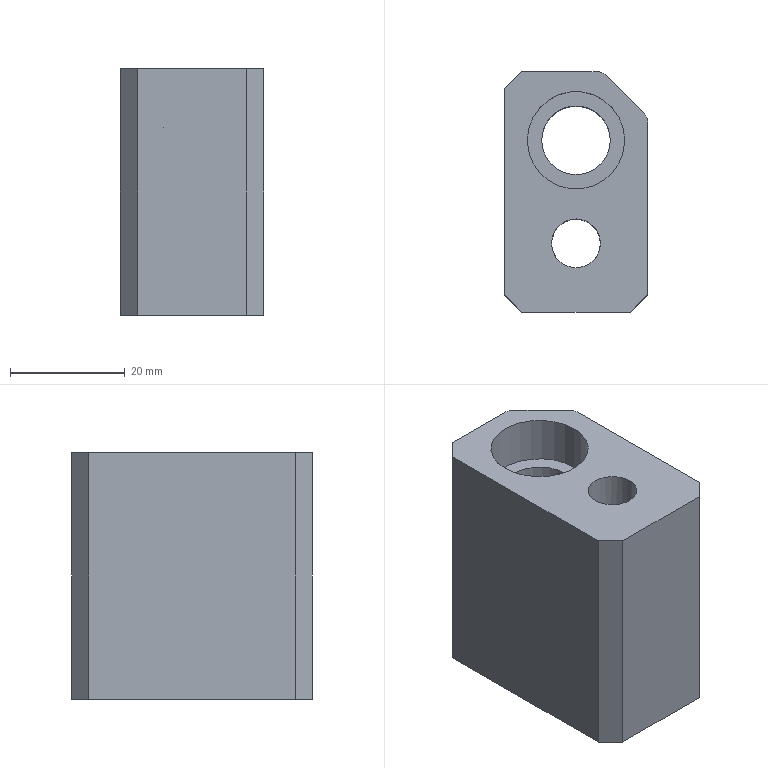Part | NX | features PH-5 2 | 1 solid | 18 faces | box 25 x 42 x 43 mm | volume 33756 mm3 | plane 12 | cylinder 6 | commonest cylinder face diameters 4 x2 8.5 x1 12.001 x1 14.5 x1 17 x1
STEP:
#1=CARTESIAN_POINT('',(2467.597,-809.449,945.716));
#2=VERTEX_POINT('',#1);
#3=CARTESIAN_POINT('',(2459.097,-809.449,945.716));
#4=DIRECTION('',(0.,0.,1.));
#5=DIRECTION('',(1.,0.,0.));
#6=AXIS2_PLACEMENT_3D('',#3,#4,#5);
#7=CIRCLE('',#6,8.5);
#8=EDGE_CURVE('',#2,#2,#7,.F.);
#9=ORIENTED_EDGE('',*,*,#8,.T.);
#10=EDGE_LOOP('',(#9));
#11=FACE_BOUND('',#10,.T.);
#12=CARTESIAN_POINT('',(2459.097,-831.699,945.716));
#13=VERTEX_POINT('',#12);
#14=CARTESIAN_POINT('',(2459.097,-827.449,945.716));
#15=DIRECTION('',(0.,0.,1.));
#16=DIRECTION('',(0.,-1.,0.));
#17=AXIS2_PLACEMENT_3D('',#14,#15,#16);
#18=CIRCLE('',#17,4.25);
#19=EDGE_CURVE('',#13,#13,#18,.T.);
#20=ORIENTED_EDGE('',*,*,#19,.F.);
#21=EDGE_LOOP('',(#20));
#22=FACE_BOUND('',#21,.T.);
#23=CARTESIAN_POINT('',(2471.011,-804.863,945.716));
#24=VERTEX_POINT('',#23);
#25=CARTESIAN_POINT('',(2464.183,-798.035,945.716));
#26=VERTEX_POINT('',#25);
#27=CARTESIAN_POINT('',(2472.347,-806.199,945.716));
#28=DIRECTION('',(0.7071,-0.7071,0.));
#29=VECTOR('',#28,1000.);
#30=LINE('',#27,#29);
#31=EDGE_CURVE('',#24,#26,#30,.F.);
#32=ORIENTED_EDGE('',*,*,#31,.T.);
#33=CARTESIAN_POINT('',(2462.769,-797.449,945.716));
#34=VERTEX_POINT('',#33);
#35=CARTESIAN_POINT('',(2462.769,-799.449,945.716));
#36=DIRECTION('',(0.,0.,1.));
#37=DIRECTION('',(1.,0.,0.));
#38=AXIS2_PLACEMENT_3D('',#35,#36,#37);
#39=CIRCLE('',#38,2.);
#40=EDGE_CURVE('',#26,#34,#39,.T.);
#41=ORIENTED_EDGE('',*,*,#40,.T.);
#42=CARTESIAN_POINT('',(2449.597,-797.449,945.716));
#43=VERTEX_POINT('',#42);
#44=CARTESIAN_POINT('',(2459.097,-797.449,945.716));
#45=DIRECTION('',(1.,0.,0.));
#46=VECTOR('',#45,1000.);
#47=LINE('',#44,#46);
#48=EDGE_CURVE('',#43,#34,#47,.T.);
#49=ORIENTED_EDGE('',*,*,#48,.F.);
#50=CARTESIAN_POINT('',(2446.597,-800.449,945.716));
#51=VERTEX_POINT('',#50);
#52=CARTESIAN_POINT('',(2443.347,-803.699,945.716));
#53=DIRECTION('',(0.7071,0.7071,0.));
#54=VECTOR('',#53,1000.);
#55=LINE('',#52,#54);
#56=EDGE_CURVE('',#43,#51,#55,.F.);
#57=ORIENTED_EDGE('',*,*,#56,.T.);
#58=CARTESIAN_POINT('',(2446.597,-836.449,945.716));
#59=VERTEX_POINT('',#58);
#60=CARTESIAN_POINT('',(2446.597,-819.449,945.716));
#61=DIRECTION('',(0.,1.,0.));
#62=VECTOR('',#61,1000.);
#63=LINE('',#60,#62);
#64=EDGE_CURVE('',#59,#51,#63,.T.);
#65=ORIENTED_EDGE('',*,*,#64,.F.);
#66=CARTESIAN_POINT('',(2449.597,-839.449,945.716));
#67=VERTEX_POINT('',#66);
#68=CARTESIAN_POINT('',(2444.347,-834.199,945.716));
#69=DIRECTION('',(-0.7071,0.7071,0.));
#70=VECTOR('',#69,1000.);
#71=LINE('',#68,#70);
#72=EDGE_CURVE('',#59,#67,#71,.F.);
#73=ORIENTED_EDGE('',*,*,#72,.T.);
#74=CARTESIAN_POINT('',(2468.597,-839.449,945.716));
#75=VERTEX_POINT('',#74);
#76=CARTESIAN_POINT('',(2459.097,-839.449,945.716));
#77=DIRECTION('',(-1.,0.,0.));
#78=VECTOR('',#77,1000.);
#79=LINE('',#76,#78);
#80=EDGE_CURVE('',#75,#67,#79,.T.);
#81=ORIENTED_EDGE('',*,*,#80,.F.);
#82=CARTESIAN_POINT('',(2471.597,-836.449,945.716));
#83=VERTEX_POINT('',#82);
#84=CARTESIAN_POINT('',(2473.847,-834.199,945.716));
#85=DIRECTION('',(-0.7071,-0.7071,0.));
#86=VECTOR('',#85,1000.);
#87=LINE('',#84,#86);
#88=EDGE_CURVE('',#75,#83,#87,.F.);
#89=ORIENTED_EDGE('',*,*,#88,.T.);
#90=CARTESIAN_POINT('',(2471.597,-806.277,945.716));
#91=VERTEX_POINT('',#90);
#92=CARTESIAN_POINT('',(2471.597,-819.449,945.716));
#93=DIRECTION('',(0.,-1.,0.));
#94=VECTOR('',#93,1000.);
#95=LINE('',#92,#94);
#96=EDGE_CURVE('',#91,#83,#95,.T.);
#97=ORIENTED_EDGE('',*,*,#96,.F.);
#98=CARTESIAN_POINT('',(2469.597,-806.277,945.716));
#99=DIRECTION('',(0.,0.,1.));
#100=DIRECTION('',(1.,0.,0.));
#101=AXIS2_PLACEMENT_3D('',#98,#99,#100);
#102=CIRCLE('',#101,2.);
#103=EDGE_CURVE('',#91,#24,#102,.T.);
#104=ORIENTED_EDGE('',*,*,#103,.T.);
#105=EDGE_LOOP('',(#32,#41,#49,#57,#65,#73,#81,#89,#97,#104));
#106=FACE_BOUND('',#105,.T.);
#107=CARTESIAN_POINT('',(2459.097,-819.449,945.716));
#108=DIRECTION('',(0.,0.,1.));
#109=DIRECTION('',(-1.,0.,0.));
#110=AXIS2_PLACEMENT_3D('',#107,#108,#109);
#111=PLANE('',#110);
#112=ADVANCED_FACE('',(#11,#22,#106),#111,.T.);
#113=ORIENTED_EDGE('',*,*,#48,.T.);
#114=CARTESIAN_POINT('',(2462.769,-797.449,902.716));
#115=VERTEX_POINT('',#114);
#116=CARTESIAN_POINT('',(2462.769,-797.449,920.716));
#117=DIRECTION('',(0.,0.,1.));
#118=VECTOR('',#117,1000.);
#119=LINE('',#116,#118);
#120=EDGE_CURVE('',#34,#115,#119,.F.);
#121=ORIENTED_EDGE('',*,*,#120,.T.);
#122=CARTESIAN_POINT('',(2449.597,-797.449,902.716));
#123=VERTEX_POINT('',#122);
#124=CARTESIAN_POINT('',(2459.097,-797.449,902.716));
#125=DIRECTION('',(-1.,0.,0.));
#126=VECTOR('',#125,1000.);
#127=LINE('',#124,#126);
#128=EDGE_CURVE('',#115,#123,#127,.T.);
#129=ORIENTED_EDGE('',*,*,#128,.T.);
#130=CARTESIAN_POINT('',(2449.597,-797.449,920.716));
#131=DIRECTION('',(0.,0.,-1.));
#132=VECTOR('',#131,1000.);
#133=LINE('',#130,#132);
#134=EDGE_CURVE('',#123,#43,#133,.F.);
#135=ORIENTED_EDGE('',*,*,#134,.T.);
#136=EDGE_LOOP('',(#113,#121,#129,#135));
#137=FACE_BOUND('',#136,.T.);
#138=CARTESIAN_POINT('',(2459.097,-797.449,920.716));
#139=DIRECTION('',(0.,1.,0.));
#140=DIRECTION('',(0.,0.,-1.));
#141=AXIS2_PLACEMENT_3D('',#138,#139,#140);
#142=PLANE('',#141);
#143=ADVANCED_FACE('',(#137),#142,.T.);
#144=CARTESIAN_POINT('',(2471.597,-836.449,902.716));
#145=VERTEX_POINT('',#144);
#146=CARTESIAN_POINT('',(2471.597,-806.277,902.716));
#147=VERTEX_POINT('',#146);
#148=CARTESIAN_POINT('',(2471.597,-819.449,902.716));
#149=DIRECTION('',(0.,1.,0.));
#150=VECTOR('',#149,1000.);
#151=LINE('',#148,#150);
#152=EDGE_CURVE('',#145,#147,#151,.T.);
#153=ORIENTED_EDGE('',*,*,#152,.T.);
#154=CARTESIAN_POINT('',(2471.597,-806.277,920.716));
#155=DIRECTION('',(0.,0.,-1.));
#156=VECTOR('',#155,1000.);
#157=LINE('',#154,#156);
#158=EDGE_CURVE('',#147,#91,#157,.F.);
#159=ORIENTED_EDGE('',*,*,#158,.T.);
#160=ORIENTED_EDGE('',*,*,#96,.T.);
#161=CARTESIAN_POINT('',(2471.597,-836.449,920.716));
#162=DIRECTION('',(0.,0.,-1.));
#163=VECTOR('',#162,1000.);
#164=LINE('',#161,#163);
#165=EDGE_CURVE('',#83,#145,#164,.T.);
#166=ORIENTED_EDGE('',*,*,#165,.T.);
#167=EDGE_LOOP('',(#153,#159,#160,#166));
#168=FACE_BOUND('',#167,.T.);
#169=CARTESIAN_POINT('',(2471.597,-819.449,920.716));
#170=DIRECTION('',(1.,0.,0.));
#171=DIRECTION('',(0.,0.,1.));
#172=AXIS2_PLACEMENT_3D('',#169,#170,#171);
#173=PLANE('',#172);
#174=ADVANCED_FACE('',(#168),#173,.T.);
#175=CARTESIAN_POINT('',(2449.597,-839.449,902.716));
#176=VERTEX_POINT('',#175);
#177=CARTESIAN_POINT('',(2468.597,-839.449,902.716));
#178=VERTEX_POINT('',#177);
#179=CARTESIAN_POINT('',(2459.097,-839.449,902.716));
#180=DIRECTION('',(1.,0.,0.));
#181=VECTOR('',#180,1000.);
#182=LINE('',#179,#181);
#183=EDGE_CURVE('',#176,#178,#182,.T.);
#184=ORIENTED_EDGE('',*,*,#183,.T.);
#185=CARTESIAN_POINT('',(2468.597,-839.449,920.716));
#186=DIRECTION('',(0.,0.,1.));
#187=VECTOR('',#186,1000.);
#188=LINE('',#185,#187);
#189=EDGE_CURVE('',#178,#75,#188,.T.);
#190=ORIENTED_EDGE('',*,*,#189,.T.);
#191=ORIENTED_EDGE('',*,*,#80,.T.);
#192=CARTESIAN_POINT('',(2449.597,-839.449,920.716));
#193=DIRECTION('',(0.,0.,-1.));
#194=VECTOR('',#193,1000.);
#195=LINE('',#192,#194);
#196=EDGE_CURVE('',#67,#176,#195,.T.);
#197=ORIENTED_EDGE('',*,*,#196,.T.);
#198=EDGE_LOOP('',(#184,#190,#191,#197));
#199=FACE_BOUND('',#198,.T.);
#200=CARTESIAN_POINT('',(2459.097,-839.449,920.716));
#201=DIRECTION('',(0.,-1.,0.));
#202=DIRECTION('',(0.,0.,1.));
#203=AXIS2_PLACEMENT_3D('',#200,#201,#202);
#204=PLANE('',#203);
#205=ADVANCED_FACE('',(#199),#204,.T.);
#206=CARTESIAN_POINT('',(2453.097,-809.449,902.716));
#207=VERTEX_POINT('',#206);
#208=CARTESIAN_POINT('',(2459.097,-809.449,902.716));
#209=DIRECTION('',(0.,0.,-1.));
#210=DIRECTION('',(-1.,0.,0.));
#211=AXIS2_PLACEMENT_3D('',#208,#209,#210);
#212=CIRCLE('',#211,6.);
#213=EDGE_CURVE('',#207,#207,#212,.T.);
#214=ORIENTED_EDGE('',*,*,#213,.F.);
#215=EDGE_LOOP('',(#214));
#216=FACE_BOUND('',#215,.T.);
#217=CARTESIAN_POINT('',(2451.847,-827.449,902.716));
#218=VERTEX_POINT('',#217);
#219=CARTESIAN_POINT('',(2459.097,-827.449,902.716));
#220=DIRECTION('',(0.,0.,-1.));
#221=DIRECTION('',(-1.,0.,0.));
#222=AXIS2_PLACEMENT_3D('',#219,#220,#221);
#223=CIRCLE('',#222,7.25);
#224=EDGE_CURVE('',#218,#218,#223,.F.);
#225=ORIENTED_EDGE('',*,*,#224,.T.);
#226=EDGE_LOOP('',(#225));
#227=FACE_BOUND('',#226,.T.);
#228=ORIENTED_EDGE('',*,*,#128,.F.);
#229=CARTESIAN_POINT('',(2464.183,-798.035,902.716));
#230=VERTEX_POINT('',#229);
#231=CARTESIAN_POINT('',(2462.769,-799.449,902.716));
#232=DIRECTION('',(0.,0.,-1.));
#233=DIRECTION('',(-1.,0.,0.));
#234=AXIS2_PLACEMENT_3D('',#231,#232,#233);
#235=CIRCLE('',#234,2.);
#236=EDGE_CURVE('',#115,#230,#235,.T.);
#237=ORIENTED_EDGE('',*,*,#236,.T.);
#238=CARTESIAN_POINT('',(2471.011,-804.863,902.716));
#239=VERTEX_POINT('',#238);
#240=CARTESIAN_POINT('',(2472.347,-806.199,902.716));
#241=DIRECTION('',(-0.7071,0.7071,0.));
#242=VECTOR('',#241,1000.);
#243=LINE('',#240,#242);
#244=EDGE_CURVE('',#230,#239,#243,.F.);
#245=ORIENTED_EDGE('',*,*,#244,.T.);
#246=CARTESIAN_POINT('',(2469.597,-806.277,902.716));
#247=DIRECTION('',(0.,0.,-1.));
#248=DIRECTION('',(-1.,0.,0.));
#249=AXIS2_PLACEMENT_3D('',#246,#247,#248);
#250=CIRCLE('',#249,2.);
#251=EDGE_CURVE('',#239,#147,#250,.T.);
#252=ORIENTED_EDGE('',*,*,#251,.T.);
#253=ORIENTED_EDGE('',*,*,#152,.F.);
#254=CARTESIAN_POINT('',(2473.847,-834.199,902.716));
#255=DIRECTION('',(0.7071,0.7071,0.));
#256=VECTOR('',#255,1000.);
#257=LINE('',#254,#256);
#258=EDGE_CURVE('',#145,#178,#257,.F.);
#259=ORIENTED_EDGE('',*,*,#258,.T.);
#260=ORIENTED_EDGE('',*,*,#183,.F.);
#261=CARTESIAN_POINT('',(2446.597,-836.449,902.716));
#262=VERTEX_POINT('',#261);
#263=CARTESIAN_POINT('',(2444.347,-834.199,902.716));
#264=DIRECTION('',(0.7071,-0.7071,0.));
#265=VECTOR('',#264,1000.);
#266=LINE('',#263,#265);
#267=EDGE_CURVE('',#176,#262,#266,.F.);
#268=ORIENTED_EDGE('',*,*,#267,.T.);
#269=CARTESIAN_POINT('',(2446.597,-800.449,902.716));
#270=VERTEX_POINT('',#269);
#271=CARTESIAN_POINT('',(2446.597,-819.449,902.716));
#272=DIRECTION('',(0.,-1.,0.));
#273=VECTOR('',#272,1000.);
#274=LINE('',#271,#273);
#275=EDGE_CURVE('',#270,#262,#274,.T.);
#276=ORIENTED_EDGE('',*,*,#275,.F.);
#277=CARTESIAN_POINT('',(2443.347,-803.699,902.716));
#278=DIRECTION('',(-0.7071,-0.7071,0.));
#279=VECTOR('',#278,1000.);
#280=LINE('',#277,#279);
#281=EDGE_CURVE('',#270,#123,#280,.F.);
#282=ORIENTED_EDGE('',*,*,#281,.T.);
#283=EDGE_LOOP('',(#228,#237,#245,#252,#253,#259,#260,#268,#276,#282));
#284=FACE_BOUND('',#283,.T.);
#285=CARTESIAN_POINT('',(2459.097,-819.449,902.716));
#286=DIRECTION('',(0.,0.,-1.));
#287=DIRECTION('',(1.,0.,0.));
#288=AXIS2_PLACEMENT_3D('',#285,#286,#287);
#289=PLANE('',#288);
#290=ADVANCED_FACE('',(#216,#227,#284),#289,.T.);
#291=ORIENTED_EDGE('',*,*,#275,.T.);
#292=CARTESIAN_POINT('',(2446.597,-836.449,920.716));
#293=DIRECTION('',(0.,0.,1.));
#294=VECTOR('',#293,1000.);
#295=LINE('',#292,#294);
#296=EDGE_CURVE('',#262,#59,#295,.T.);
#297=ORIENTED_EDGE('',*,*,#296,.T.);
#298=ORIENTED_EDGE('',*,*,#64,.T.);
#299=CARTESIAN_POINT('',(2446.597,-800.449,920.716));
#300=DIRECTION('',(0.,0.,1.));
#301=VECTOR('',#300,1000.);
#302=LINE('',#299,#301);
#303=EDGE_CURVE('',#51,#270,#302,.F.);
#304=ORIENTED_EDGE('',*,*,#303,.T.);
#305=EDGE_LOOP('',(#291,#297,#298,#304));
#306=FACE_BOUND('',#305,.T.);
#307=CARTESIAN_POINT('',(2446.597,-819.449,920.716));
#308=DIRECTION('',(-1.,0.,0.));
#309=DIRECTION('',(0.,0.,-1.));
#310=AXIS2_PLACEMENT_3D('',#307,#308,#309);
#311=PLANE('',#310);
#312=ADVANCED_FACE('',(#306),#311,.T.);
#313=ORIENTED_EDGE('',*,*,#267,.F.);
#314=ORIENTED_EDGE('',*,*,#196,.F.);
#315=ORIENTED_EDGE('',*,*,#72,.F.);
#316=ORIENTED_EDGE('',*,*,#296,.F.);
#317=EDGE_LOOP('',(#313,#314,#315,#316));
#318=FACE_BOUND('',#317,.T.);
#319=CARTESIAN_POINT('',(2446.597,-836.449,920.716));
#320=DIRECTION('',(0.7071,0.7071,0.));
#321=DIRECTION('',(-0.7071,0.7071,0.));
#322=AXIS2_PLACEMENT_3D('',#319,#320,#321);
#323=PLANE('',#322);
#324=ADVANCED_FACE('',(#318),#323,.F.);
#325=ORIENTED_EDGE('',*,*,#281,.F.);
#326=ORIENTED_EDGE('',*,*,#303,.F.);
#327=ORIENTED_EDGE('',*,*,#56,.F.);
#328=ORIENTED_EDGE('',*,*,#134,.F.);
#329=EDGE_LOOP('',(#325,#326,#327,#328));
#330=FACE_BOUND('',#329,.T.);
#331=CARTESIAN_POINT('',(2449.597,-797.449,920.716));
#332=DIRECTION('',(0.7071,-0.7071,0.));
#333=DIRECTION('',(0.7071,0.7071,0.));
#334=AXIS2_PLACEMENT_3D('',#331,#332,#333);
#335=PLANE('',#334);
#336=ADVANCED_FACE('',(#330),#335,.F.);
#337=CARTESIAN_POINT('',(2463.347,-827.449,913.716));
#338=VERTEX_POINT('',#337);
#339=CARTESIAN_POINT('',(2459.097,-827.449,913.716));
#340=DIRECTION('',(0.,0.,1.));
#341=DIRECTION('',(1.,0.,0.));
#342=AXIS2_PLACEMENT_3D('',#339,#340,#341);
#343=CIRCLE('',#342,4.25);
#344=EDGE_CURVE('',#338,#338,#343,.T.);
#345=ORIENTED_EDGE('',*,*,#344,.T.);
#346=EDGE_LOOP('',(#345));
#347=FACE_BOUND('',#346,.T.);
#348=CARTESIAN_POINT('',(2466.347,-827.449,913.716));
#349=VERTEX_POINT('',#348);
#350=CARTESIAN_POINT('',(2459.097,-827.449,913.716));
#351=DIRECTION('',(0.,0.,1.));
#352=DIRECTION('',(1.,0.,0.));
#353=AXIS2_PLACEMENT_3D('',#350,#351,#352);
#354=CIRCLE('',#353,7.25);
#355=EDGE_CURVE('',#349,#349,#354,.T.);
#356=ORIENTED_EDGE('',*,*,#355,.F.);
#357=EDGE_LOOP('',(#356));
#358=FACE_BOUND('',#357,.T.);
#359=CARTESIAN_POINT('',(2459.097,-827.449,913.716));
#360=DIRECTION('',(0.,0.,1.));
#361=DIRECTION('',(0.,-1.,0.));
#362=AXIS2_PLACEMENT_3D('',#359,#360,#361);
#363=PLANE('',#362);
#364=ADVANCED_FACE('',(#347,#358),#363,.F.);
#365=ORIENTED_EDGE('',*,*,#224,.F.);
#366=EDGE_LOOP('',(#365));
#367=FACE_BOUND('',#366,.T.);
#368=ORIENTED_EDGE('',*,*,#355,.T.);
#369=EDGE_LOOP('',(#368));
#370=FACE_BOUND('',#369,.T.);
#371=CARTESIAN_POINT('',(2459.097,-827.449,931.716));
#372=DIRECTION('',(0.,0.,-1.));
#373=DIRECTION('',(-1.,0.,0.));
#374=AXIS2_PLACEMENT_3D('',#371,#372,#373);
#375=CYLINDRICAL_SURFACE('',#374,7.25);
#376=ADVANCED_FACE('',(#367,#370),#375,.F.);
#377=ORIENTED_EDGE('',*,*,#19,.T.);
#378=EDGE_LOOP('',(#377));
#379=FACE_BOUND('',#378,.T.);
#380=ORIENTED_EDGE('',*,*,#344,.F.);
#381=EDGE_LOOP('',(#380));
#382=FACE_BOUND('',#381,.T.);
#383=CARTESIAN_POINT('',(2459.097,-827.449,946.716));
#384=DIRECTION('',(0.,0.,-1.));
#385=DIRECTION('',(-1.,0.,0.));
#386=AXIS2_PLACEMENT_3D('',#383,#384,#385);
#387=CYLINDRICAL_SURFACE('',#386,4.25);
#388=ADVANCED_FACE('',(#379,#382),#387,.F.);
#389=ORIENTED_EDGE('',*,*,#213,.T.);
#390=EDGE_LOOP('',(#389));
#391=FACE_BOUND('',#390,.T.);
#392=CARTESIAN_POINT('',(2453.097,-809.449,937.516));
#393=VERTEX_POINT('',#392);
#394=CARTESIAN_POINT('',(2459.097,-809.449,937.516));
#395=DIRECTION('',(0.,0.,-1.));
#396=DIRECTION('',(-1.,0.,0.));
#397=AXIS2_PLACEMENT_3D('',#394,#395,#396);
#398=CIRCLE('',#397,6.);
#399=EDGE_CURVE('',#393,#393,#398,.T.);
#400=ORIENTED_EDGE('',*,*,#399,.F.);
#401=EDGE_LOOP('',(#400));
#402=FACE_BOUND('',#401,.T.);
#403=CARTESIAN_POINT('',(2459.097,-809.449,945.716));
#404=DIRECTION('',(0.,0.,-1.));
#405=DIRECTION('',(0.,-1.,0.));
#406=AXIS2_PLACEMENT_3D('',#403,#404,#405);
#407=CYLINDRICAL_SURFACE('',#406,6.);
#408=ADVANCED_FACE('',(#391,#402),#407,.F.);
#409=ORIENTED_EDGE('',*,*,#399,.T.);
#410=EDGE_LOOP('',(#409));
#411=FACE_BOUND('',#410,.T.);
#412=CARTESIAN_POINT('',(2450.597,-809.449,937.516));
#413=VERTEX_POINT('',#412);
#414=CARTESIAN_POINT('',(2459.097,-809.449,937.516));
#415=DIRECTION('',(0.,0.,-1.));
#416=DIRECTION('',(-1.,0.,0.));
#417=AXIS2_PLACEMENT_3D('',#414,#415,#416);
#418=CIRCLE('',#417,8.5);
#419=EDGE_CURVE('',#413,#413,#418,.T.);
#420=ORIENTED_EDGE('',*,*,#419,.F.);
#421=EDGE_LOOP('',(#420));
#422=FACE_BOUND('',#421,.T.);
#423=CARTESIAN_POINT('',(2459.097,-809.449,937.516));
#424=DIRECTION('',(0.,0.,-1.));
#425=DIRECTION('',(0.,1.,0.));
#426=AXIS2_PLACEMENT_3D('',#423,#424,#425);
#427=PLANE('',#426);
#428=ADVANCED_FACE('',(#411,#422),#427,.F.);
#429=ORIENTED_EDGE('',*,*,#419,.T.);
#430=EDGE_LOOP('',(#429));
#431=FACE_BOUND('',#430,.T.);
#432=ORIENTED_EDGE('',*,*,#8,.F.);
#433=EDGE_LOOP('',(#432));
#434=FACE_BOUND('',#433,.T.);
#435=CARTESIAN_POINT('',(2459.097,-809.449,945.716));
#436=DIRECTION('',(0.,0.,-1.));
#437=DIRECTION('',(0.,-1.,0.));
#438=AXIS2_PLACEMENT_3D('',#435,#436,#437);
#439=CYLINDRICAL_SURFACE('',#438,8.5);
#440=ADVANCED_FACE('',(#431,#434),#439,.F.);
#441=ORIENTED_EDGE('',*,*,#88,.F.);
#442=ORIENTED_EDGE('',*,*,#189,.F.);
#443=ORIENTED_EDGE('',*,*,#258,.F.);
#444=ORIENTED_EDGE('',*,*,#165,.F.);
#445=EDGE_LOOP('',(#441,#442,#443,#444));
#446=FACE_BOUND('',#445,.T.);
#447=CARTESIAN_POINT('',(2471.597,-836.449,920.716));
#448=DIRECTION('',(-0.7071,0.7071,0.));
#449=DIRECTION('',(0.,0.,-1.));
#450=AXIS2_PLACEMENT_3D('',#447,#448,#449);
#451=PLANE('',#450);
#452=ADVANCED_FACE('',(#446),#451,.F.);
#453=ORIENTED_EDGE('',*,*,#244,.F.);
#454=CARTESIAN_POINT('',(2464.183,-798.035,920.716));
#455=DIRECTION('',(0.,0.,-1.));
#456=VECTOR('',#455,1000.);
#457=LINE('',#454,#456);
#458=EDGE_CURVE('',#230,#26,#457,.F.);
#459=ORIENTED_EDGE('',*,*,#458,.T.);
#460=ORIENTED_EDGE('',*,*,#31,.F.);
#461=CARTESIAN_POINT('',(2471.011,-804.863,920.716));
#462=DIRECTION('',(0.,0.,1.));
#463=VECTOR('',#462,1000.);
#464=LINE('',#461,#463);
#465=EDGE_CURVE('',#24,#239,#464,.F.);
#466=ORIENTED_EDGE('',*,*,#465,.T.);
#467=EDGE_LOOP('',(#453,#459,#460,#466));
#468=FACE_BOUND('',#467,.T.);
#469=CARTESIAN_POINT('',(2463.597,-797.449,920.716));
#470=DIRECTION('',(-0.7071,-0.7071,0.));
#471=DIRECTION('',(0.,0.,-1.));
#472=AXIS2_PLACEMENT_3D('',#469,#470,#471);
#473=PLANE('',#472);
#474=ADVANCED_FACE('',(#468),#473,.F.);
#475=ORIENTED_EDGE('',*,*,#40,.F.);
#476=ORIENTED_EDGE('',*,*,#458,.F.);
#477=ORIENTED_EDGE('',*,*,#236,.F.);
#478=ORIENTED_EDGE('',*,*,#120,.F.);
#479=EDGE_LOOP('',(#475,#476,#477,#478));
#480=FACE_BOUND('',#479,.T.);
#481=CARTESIAN_POINT('',(2462.769,-799.449,920.716));
#482=DIRECTION('',(0.,0.,1.));
#483=DIRECTION('',(1.,0.,0.));
#484=AXIS2_PLACEMENT_3D('',#481,#482,#483);
#485=CYLINDRICAL_SURFACE('',#484,2.);
#486=ADVANCED_FACE('',(#480),#485,.T.);
#487=ORIENTED_EDGE('',*,*,#251,.F.);
#488=ORIENTED_EDGE('',*,*,#465,.F.);
#489=ORIENTED_EDGE('',*,*,#103,.F.);
#490=ORIENTED_EDGE('',*,*,#158,.F.);
#491=EDGE_LOOP('',(#487,#488,#489,#490));
#492=FACE_BOUND('',#491,.T.);
#493=CARTESIAN_POINT('',(2469.597,-806.277,920.716));
#494=DIRECTION('',(0.,0.,-1.));
#495=DIRECTION('',(-1.,0.,0.));
#496=AXIS2_PLACEMENT_3D('',#493,#494,#495);
#497=CYLINDRICAL_SURFACE('',#496,2.);
#498=ADVANCED_FACE('',(#492),#497,.T.);
#499=CLOSED_SHELL('',(#112,#143,#174,#205,#290,#312,#324,#336,#364,#376,#388,#408,#428,#440,#452,#474,#486,#498));
#500=MANIFOLD_SOLID_BREP('',#499);
#501=(LENGTH_UNIT()NAMED_UNIT(*)SI_UNIT(.MILLI.,.METRE.));
#502=UNCERTAINTY_MEASURE_WITH_UNIT(LENGTH_MEASURE(0.00001),#501,'','');
#503=(NAMED_UNIT(*)PLANE_ANGLE_UNIT()SI_UNIT($,.RADIAN.));
#504=(NAMED_UNIT(*)SI_UNIT($,.STERADIAN.)SOLID_ANGLE_UNIT());
#505=(GEOMETRIC_REPRESENTATION_CONTEXT(3)GLOBAL_UNCERTAINTY_ASSIGNED_CONTEXT((#502))GLOBAL_UNIT_ASSIGNED_CONTEXT((#501,#503,#504))REPRESENTATION_CONTEXT('',''));
#506=ADVANCED_BREP_SHAPE_REPRESENTATION('',(#500),#505);